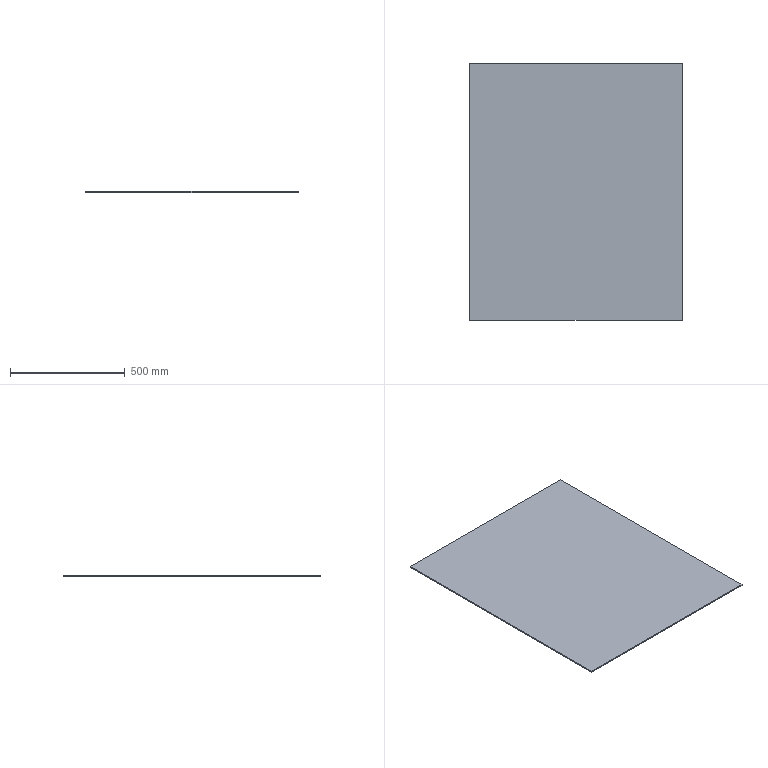Part | SolidWorks | features Extrusion 1 | 1 solid | 6 faces | box 926 x 1119 x 5 mm | volume 5180970 mm3 | plane 6
STEP:
#1=CARTESIAN_POINT('',(463.,-559.5,0.));
#2=VERTEX_POINT('',#1);
#3=CARTESIAN_POINT('',(463.,559.5,0.));
#4=VERTEX_POINT('',#3);
#5=CARTESIAN_POINT('',(463.,559.5,0.));
#6=DIRECTION('',(0.,1.,0.));
#7=VECTOR('',#6,1000.);
#8=LINE('',#5,#7);
#9=EDGE_CURVE('',#2,#4,#8,.T.);
#10=ORIENTED_EDGE('',*,*,#9,.T.);
#11=CARTESIAN_POINT('',(463.,559.5,5.));
#12=VERTEX_POINT('',#11);
#13=CARTESIAN_POINT('',(463.,559.5,5.));
#14=DIRECTION('',(0.,0.,-1.));
#15=VECTOR('',#14,1000.);
#16=LINE('',#13,#15);
#17=EDGE_CURVE('',#12,#4,#16,.T.);
#18=ORIENTED_EDGE('',*,*,#17,.F.);
#19=CARTESIAN_POINT('',(463.,-559.5,5.));
#20=VERTEX_POINT('',#19);
#21=CARTESIAN_POINT('',(463.,559.5,5.));
#22=DIRECTION('',(0.,1.,0.));
#23=VECTOR('',#22,1000.);
#24=LINE('',#21,#23);
#25=EDGE_CURVE('',#20,#12,#24,.T.);
#26=ORIENTED_EDGE('',*,*,#25,.F.);
#27=CARTESIAN_POINT('',(463.,-559.5,5.));
#28=DIRECTION('',(0.,0.,-1.));
#29=VECTOR('',#28,1000.);
#30=LINE('',#27,#29);
#31=EDGE_CURVE('',#20,#2,#30,.T.);
#32=ORIENTED_EDGE('',*,*,#31,.T.);
#33=EDGE_LOOP('',(#10,#18,#26,#32));
#34=FACE_OUTER_BOUND('',#33,.T.);
#35=CARTESIAN_POINT('',(463.,559.5,5.));
#36=DIRECTION('',(-1.,0.,0.));
#37=DIRECTION('',(0.,-1.,0.));
#38=AXIS2_PLACEMENT_3D('',#35,#36,#37);
#39=PLANE('',#38);
#40=ADVANCED_FACE('',(#34),#39,.F.);
#41=CARTESIAN_POINT('',(-463.,559.5,0.));
#42=VERTEX_POINT('',#41);
#43=CARTESIAN_POINT('',(-463.,559.5,0.));
#44=DIRECTION('',(-1.,0.,0.));
#45=VECTOR('',#44,1000.);
#46=LINE('',#43,#45);
#47=EDGE_CURVE('',#4,#42,#46,.T.);
#48=ORIENTED_EDGE('',*,*,#47,.T.);
#49=CARTESIAN_POINT('',(-463.,559.5,5.));
#50=VERTEX_POINT('',#49);
#51=CARTESIAN_POINT('',(-463.,559.5,5.));
#52=DIRECTION('',(0.,0.,-1.));
#53=VECTOR('',#52,1000.);
#54=LINE('',#51,#53);
#55=EDGE_CURVE('',#50,#42,#54,.T.);
#56=ORIENTED_EDGE('',*,*,#55,.F.);
#57=CARTESIAN_POINT('',(-463.,559.5,5.));
#58=DIRECTION('',(-1.,0.,0.));
#59=VECTOR('',#58,1000.);
#60=LINE('',#57,#59);
#61=EDGE_CURVE('',#12,#50,#60,.T.);
#62=ORIENTED_EDGE('',*,*,#61,.F.);
#63=ORIENTED_EDGE('',*,*,#17,.T.);
#64=EDGE_LOOP('',(#48,#56,#62,#63));
#65=FACE_OUTER_BOUND('',#64,.T.);
#66=CARTESIAN_POINT('',(-463.,559.5,5.));
#67=DIRECTION('',(0.,-1.,0.));
#68=DIRECTION('',(0.,0.,-1.));
#69=AXIS2_PLACEMENT_3D('',#66,#67,#68);
#70=PLANE('',#69);
#71=ADVANCED_FACE('',(#65),#70,.F.);
#72=CARTESIAN_POINT('',(-463.,-559.5,0.));
#73=VERTEX_POINT('',#72);
#74=CARTESIAN_POINT('',(-463.,559.5,0.));
#75=DIRECTION('',(0.,-1.,0.));
#76=VECTOR('',#75,1000.);
#77=LINE('',#74,#76);
#78=EDGE_CURVE('',#42,#73,#77,.T.);
#79=ORIENTED_EDGE('',*,*,#78,.T.);
#80=CARTESIAN_POINT('',(-463.,-559.5,5.));
#81=VERTEX_POINT('',#80);
#82=CARTESIAN_POINT('',(-463.,-559.5,5.));
#83=DIRECTION('',(0.,0.,-1.));
#84=VECTOR('',#83,1000.);
#85=LINE('',#82,#84);
#86=EDGE_CURVE('',#81,#73,#85,.T.);
#87=ORIENTED_EDGE('',*,*,#86,.F.);
#88=CARTESIAN_POINT('',(-463.,559.5,5.));
#89=DIRECTION('',(0.,-1.,0.));
#90=VECTOR('',#89,1000.);
#91=LINE('',#88,#90);
#92=EDGE_CURVE('',#50,#81,#91,.T.);
#93=ORIENTED_EDGE('',*,*,#92,.F.);
#94=ORIENTED_EDGE('',*,*,#55,.T.);
#95=EDGE_LOOP('',(#79,#87,#93,#94));
#96=FACE_OUTER_BOUND('',#95,.T.);
#97=CARTESIAN_POINT('',(-463.,559.5,5.));
#98=DIRECTION('',(1.,0.,0.));
#99=DIRECTION('',(0.,1.,0.));
#100=AXIS2_PLACEMENT_3D('',#97,#98,#99);
#101=PLANE('',#100);
#102=ADVANCED_FACE('',(#96),#101,.F.);
#103=CARTESIAN_POINT('',(-463.,-559.5,0.));
#104=DIRECTION('',(1.,0.,0.));
#105=VECTOR('',#104,1000.);
#106=LINE('',#103,#105);
#107=EDGE_CURVE('',#73,#2,#106,.T.);
#108=ORIENTED_EDGE('',*,*,#107,.T.);
#109=ORIENTED_EDGE('',*,*,#31,.F.);
#110=CARTESIAN_POINT('',(-463.,-559.5,5.));
#111=DIRECTION('',(1.,0.,0.));
#112=VECTOR('',#111,1000.);
#113=LINE('',#110,#112);
#114=EDGE_CURVE('',#81,#20,#113,.T.);
#115=ORIENTED_EDGE('',*,*,#114,.F.);
#116=ORIENTED_EDGE('',*,*,#86,.T.);
#117=EDGE_LOOP('',(#108,#109,#115,#116));
#118=FACE_OUTER_BOUND('',#117,.T.);
#119=CARTESIAN_POINT('',(-463.,-559.5,5.));
#120=DIRECTION('',(0.,1.,0.));
#121=DIRECTION('',(0.,0.,1.));
#122=AXIS2_PLACEMENT_3D('',#119,#120,#121);
#123=PLANE('',#122);
#124=ADVANCED_FACE('',(#118),#123,.F.);
#125=ORIENTED_EDGE('',*,*,#25,.T.);
#126=ORIENTED_EDGE('',*,*,#61,.T.);
#127=ORIENTED_EDGE('',*,*,#92,.T.);
#128=ORIENTED_EDGE('',*,*,#114,.T.);
#129=EDGE_LOOP('',(#125,#126,#127,#128));
#130=FACE_OUTER_BOUND('',#129,.T.);
#131=CARTESIAN_POINT('',(0.,0.,5.));
#132=DIRECTION('',(0.,0.,1.));
#133=DIRECTION('',(1.,0.,0.));
#134=AXIS2_PLACEMENT_3D('',#131,#132,#133);
#135=PLANE('',#134);
#136=ADVANCED_FACE('',(#130),#135,.T.);
#137=ORIENTED_EDGE('',*,*,#9,.F.);
#138=ORIENTED_EDGE('',*,*,#107,.F.);
#139=ORIENTED_EDGE('',*,*,#78,.F.);
#140=ORIENTED_EDGE('',*,*,#47,.F.);
#141=EDGE_LOOP('',(#137,#138,#139,#140));
#142=FACE_OUTER_BOUND('',#141,.T.);
#143=CARTESIAN_POINT('',(0.,0.,0.));
#144=DIRECTION('',(0.,0.,1.));
#145=DIRECTION('',(1.,0.,0.));
#146=AXIS2_PLACEMENT_3D('',#143,#144,#145);
#147=PLANE('',#146);
#148=ADVANCED_FACE('',(#142),#147,.F.);
#149=CLOSED_SHELL('',(#40,#71,#102,#124,#136,#148));
#150=MANIFOLD_SOLID_BREP('',#149);
#151=CARTESIAN_POINT('',(0.,0.,0.));
#152=DIRECTION('',(0.,0.,1.));
#153=DIRECTION('',(1.,0.,0.));
#154=AXIS2_PLACEMENT_3D('',#151,#152,#153);
#155=(LENGTH_UNIT()NAMED_UNIT(*)SI_UNIT(.MILLI.,.METRE.));
#156=UNCERTAINTY_MEASURE_WITH_UNIT(LENGTH_MEASURE(0.00001),#155,'','');
#157=(NAMED_UNIT(*)PLANE_ANGLE_UNIT()SI_UNIT($,.RADIAN.));
#158=(NAMED_UNIT(*)SI_UNIT($,.STERADIAN.)SOLID_ANGLE_UNIT());
#159=(GEOMETRIC_REPRESENTATION_CONTEXT(3)GLOBAL_UNCERTAINTY_ASSIGNED_CONTEXT((#156))GLOBAL_UNIT_ASSIGNED_CONTEXT((#155,#157,#158))REPRESENTATION_CONTEXT('',''));
#160=ADVANCED_BREP_SHAPE_REPRESENTATION('',(#150,#154),#159);